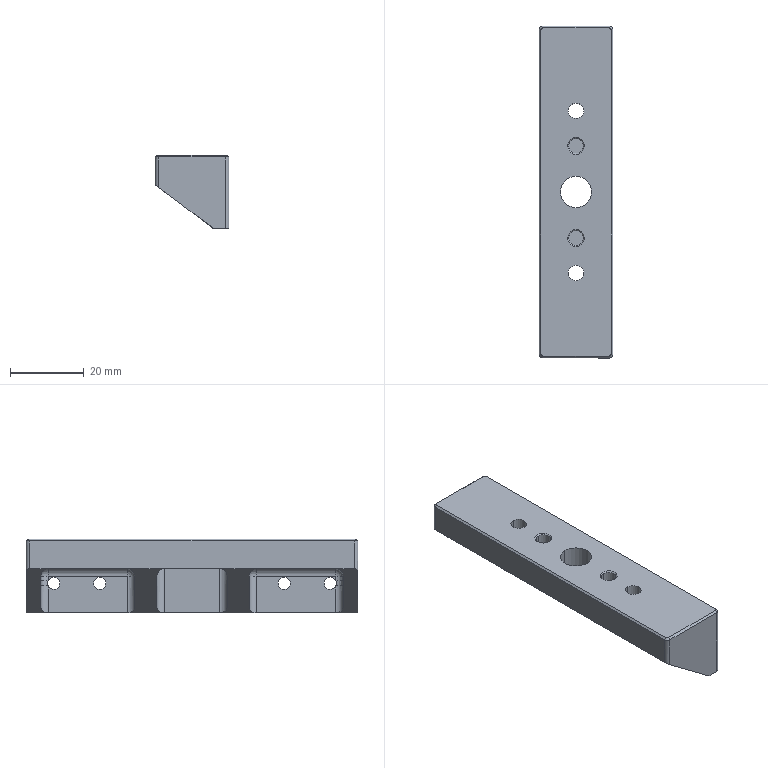NC program | NX | posted with a generic post | part box 20 x 90 x 20 mm
Whole program, first 1403 of 1621 lines:
N10 G17 G21 G94 G90
(FLOOR_WALL , TOOL : D80)
N12 T19 M6
N14 G54
N16 G17 G0 G90 X90. Y0. B0. C0. S6500 M3
N18 G43 Z30. H19
N20 Z3.
N22 G94 G1 Z0. F1500.
N24 X87.
N26 X-87.
N28 X-90.
N30 Z3.
N32 G0 Z30.
N34 M5
(DRILLING , TOOL : D6A45)
N36 T01 M6
N38 G54
N40 G17 G0 G90 X-22. Y0. B0. C0. S5000 M3
N42 G43 Z30. H1
N44 G94 G81 G98 Z-1. F350. R3.
N46 X-12.5
N48 X0.
N50 X12.5
N52 X22.
N54 G80
N56 G0 X22. Y0. Z30.
N58 M5
(DRILLING_COPY_COPY , TOOL : 4.2ZT)
N60 T04 M6
N62 G54
N64 G17 G0 G90 X-22. Y0. B0. C0. S2000 M3
N66 G43 Z30. H4
N68 G94 G83 G98 Z-10.762 F300. Q2. R3.
N70 X22.
N72 G80
N74 G0 X22. Y0. Z30.
N76 M5
(DRILLING_COPY_COPY_1_COPY , TOOL : 3.8ZT)
N78 T18 M6
N80 G54
N82 G17 G0 G90 X12.5 Y0. B0. C0. S2000 M3
N84 G43 Z30. H18
N86 G94 G83 G98 Z-7.142 F200. Q2. R3.
N88 X-12.5
N90 G80
N92 G0 X-12.5 Y0. Z30.
N94 M5
(DRILLING_COPY_COPY_COPY , TOOL : 8.5ZT)
N96 T16 M6
N98 G54
N100 G17 G0 G90 X0. Y0. B0. C0. S2000 M3
N102 G43 Z30. H16
N104 G94 G83 G98 Z-12.054 F300. Q2. R3.
N106 G80
N108 G0 X0. Y0. Z30.
N110 M5
(ZLEVEL_PROFILE , TOOL : D10)
N112 T15 M6
N114 G54
N116 G17 G0 G90 X47.475 Y-14.013 B0. C0. S9500 M3
N118 G43 Z30. H15
N120 Z1.5
N122 G94 G1 X46.237 Y-14.707 Z1.426 F1000.
N124 X44.606 Y-15.1 Z1.338
N126 X0. Z-1.
N128 X-44. F3000.
N130 G2 X-50.1 Y-9. R6.1
N132 G1 Y9.
N134 G2 X-44. Y15.1 R6.1
N136 G1 X44.
N138 G2 X50.1 Y9. R6.1
N140 G1 Y-9.
N142 G2 X44. Y-15.1 R6.1
N144 G1 X0.
N146 X-44. Z-1.176
N148 X-44.598 Y-15.071 Z-1.178
N150 X-45.19 Y-14.983 Z-1.181
N152 X-45.771 Y-14.837 Z-1.183
N154 X-46.334 Y-14.636 Z-1.185
N156 X-46.876 Y-14.38 Z-1.188
N158 X-47.389 Y-14.072 Z-1.19
N160 X-47.87 Y-13.715 Z-1.193
N162 X-48.313 Y-13.313 Z-1.195
N164 X-48.715 Y-12.87 Z-1.197
N166 X-49.072 Y-12.389 Z-1.2
N168 X-49.38 Y-11.876 Z-1.202
N170 X-49.636 Y-11.334 Z-1.204
N172 X-49.837 Y-10.771 Z-1.207
N174 X-49.983 Y-10.19 Z-1.209
N176 X-50.071 Y-9.598 Z-1.212
N178 X-50.1 Y-9. Z-1.214
N180 Y9. Z-1.286
N182 X-50.071 Y9.598 Z-1.288
N184 X-49.983 Y10.19 Z-1.291
N186 X-49.837 Y10.771 Z-1.293
N188 X-49.636 Y11.334 Z-1.296
N190 X-49.38 Y11.876 Z-1.298
N192 X-49.072 Y12.389 Z-1.3
N194 X-48.715 Y12.87 Z-1.303
N196 X-48.313 Y13.313 Z-1.305
N198 X-47.87 Y13.715 Z-1.307
N200 X-47.389 Y14.072 Z-1.31
N202 X-46.876 Y14.38 Z-1.312
N204 X-46.334 Y14.636 Z-1.315
N206 X-45.771 Y14.837 Z-1.317
N208 X-45.19 Y14.983 Z-1.319
N210 X-44.598 Y15.071 Z-1.322
N212 X-44. Y15.1 Z-1.324
N214 X34.222 Z-1.637
N216 X39.111 Z-1.656
N218 X44. Z-1.676
N220 X44.598 Y15.071 Z-1.678
N222 X45.19 Y14.983 Z-1.681
N224 X45.771 Y14.837 Z-1.683
N226 X46.334 Y14.636 Z-1.685
N228 X46.876 Y14.38 Z-1.688
N230 X47.389 Y14.072 Z-1.69
N232 X47.87 Y13.715 Z-1.693
N234 X48.313 Y13.313 Z-1.695
N236 X48.715 Y12.87 Z-1.697
N238 X49.072 Y12.389 Z-1.7
N240 X49.38 Y11.876 Z-1.702
N242 X49.636 Y11.334 Z-1.704
N244 X49.837 Y10.771 Z-1.707
N246 X49.983 Y10.19 Z-1.709
N248 X50.071 Y9.598 Z-1.712
N250 X50.1 Y9. Z-1.714
N252 Y-9. Z-1.786
N254 X50.071 Y-9.598 Z-1.788
N256 X49.983 Y-10.19 Z-1.791
N258 X49.837 Y-10.771 Z-1.793
N260 X49.636 Y-11.334 Z-1.796
N262 X49.38 Y-11.876 Z-1.798
N264 X49.072 Y-12.389 Z-1.8
N266 X48.715 Y-12.87 Z-1.803
N268 X48.313 Y-13.313 Z-1.805
N270 X47.87 Y-13.715 Z-1.807
N272 X47.389 Y-14.072 Z-1.81
N274 X46.876 Y-14.38 Z-1.812
N276 X46.334 Y-14.636 Z-1.815
N278 X45.771 Y-14.837 Z-1.817
N280 X45.19 Y-14.983 Z-1.819
N282 X44.598 Y-15.071 Z-1.822
N284 X44. Y-15.1 Z-1.824
N286 X0. Z-2.
N288 X-44. Z-2.176
N290 X-44.598 Y-15.071 Z-2.178
N292 X-45.19 Y-14.983 Z-2.181
N294 X-45.771 Y-14.837 Z-2.183
N296 X-46.334 Y-14.636 Z-2.185
N298 X-46.876 Y-14.38 Z-2.188
N300 X-47.389 Y-14.072 Z-2.19
N302 X-47.87 Y-13.715 Z-2.193
N304 X-48.313 Y-13.313 Z-2.195
N306 X-48.715 Y-12.87 Z-2.197
N308 X-49.072 Y-12.389 Z-2.2
N310 X-49.38 Y-11.876 Z-2.202
N312 X-49.636 Y-11.334 Z-2.204
N314 X-49.837 Y-10.771 Z-2.207
N316 X-49.983 Y-10.19 Z-2.209
N318 X-50.071 Y-9.598 Z-2.212
N320 X-50.1 Y-9. Z-2.214
N322 Y9. Z-2.286
N324 X-50.071 Y9.598 Z-2.288
N326 X-49.983 Y10.19 Z-2.291
N328 X-49.837 Y10.771 Z-2.293
N330 X-49.636 Y11.334 Z-2.296
N332 X-49.38 Y11.876 Z-2.298
N334 X-49.072 Y12.389 Z-2.3
N336 X-48.715 Y12.87 Z-2.303
N338 X-48.313 Y13.313 Z-2.305
N340 X-47.87 Y13.715 Z-2.307
N342 X-47.389 Y14.072 Z-2.31
N344 X-46.876 Y14.38 Z-2.312
N346 X-46.334 Y14.636 Z-2.315
N348 X-45.771 Y14.837 Z-2.317
N350 X-45.19 Y14.983 Z-2.319
N352 X-44.598 Y15.071 Z-2.322
N354 X-44. Y15.1 Z-2.324
N356 X34.222 Z-2.637
N358 X39.111 Z-2.656
N360 X44. Z-2.676
N362 X44.598 Y15.071 Z-2.678
N364 X45.19 Y14.983 Z-2.681
N366 X45.771 Y14.837 Z-2.683
N368 X46.334 Y14.636 Z-2.685
N370 X46.876 Y14.38 Z-2.688
N372 X47.389 Y14.072 Z-2.69
N374 X47.87 Y13.715 Z-2.693
N376 X48.313 Y13.313 Z-2.695
N378 X48.715 Y12.87 Z-2.697
N380 X49.072 Y12.389 Z-2.7
N382 X49.38 Y11.876 Z-2.702
N384 X49.636 Y11.334 Z-2.704
N386 X49.837 Y10.771 Z-2.707
N388 X49.983 Y10.19 Z-2.709
N390 X50.071 Y9.598 Z-2.712
N392 X50.1 Y9. Z-2.714
N394 Y-9. Z-2.786
N396 X50.071 Y-9.598 Z-2.788
N398 X49.983 Y-10.19 Z-2.791
N400 X49.837 Y-10.771 Z-2.793
N402 X49.636 Y-11.334 Z-2.796
N404 X49.38 Y-11.876 Z-2.798
N406 X49.072 Y-12.389 Z-2.8
N408 X48.715 Y-12.87 Z-2.803
N410 X48.313 Y-13.313 Z-2.805
N412 X47.87 Y-13.715 Z-2.807
N414 X47.389 Y-14.072 Z-2.81
N416 X46.876 Y-14.38 Z-2.812
N418 X46.334 Y-14.636 Z-2.815
N420 X45.771 Y-14.837 Z-2.817
N422 X45.19 Y-14.983 Z-2.819
N424 X44.598 Y-15.071 Z-2.822
N426 X44. Y-15.1 Z-2.824
N428 X0. Z-3.
N430 X-44. Z-3.176
N432 X-44.598 Y-15.071 Z-3.178
N434 X-45.19 Y-14.983 Z-3.181
N436 X-45.771 Y-14.837 Z-3.183
N438 X-46.334 Y-14.636 Z-3.185
N440 X-46.876 Y-14.38 Z-3.188
N442 X-47.389 Y-14.072 Z-3.19
N444 X-47.87 Y-13.715 Z-3.193
N446 X-48.313 Y-13.313 Z-3.195
N448 X-48.715 Y-12.87 Z-3.197
N450 X-49.072 Y-12.389 Z-3.2
N452 X-49.38 Y-11.876 Z-3.202
N454 X-49.636 Y-11.334 Z-3.204
N456 X-49.837 Y-10.771 Z-3.207
N458 X-49.983 Y-10.19 Z-3.209
N460 X-50.071 Y-9.598 Z-3.212
N462 X-50.1 Y-9. Z-3.214
N464 Y9. Z-3.286
N466 X-50.071 Y9.598 Z-3.288
N468 X-49.983 Y10.19 Z-3.291
N470 X-49.837 Y10.771 Z-3.293
N472 X-49.636 Y11.334 Z-3.296
N474 X-49.38 Y11.876 Z-3.298
N476 X-49.072 Y12.389 Z-3.3
N478 X-48.715 Y12.87 Z-3.303
N480 X-48.313 Y13.313 Z-3.305
N482 X-47.87 Y13.715 Z-3.307
N484 X-47.389 Y14.072 Z-3.31
N486 X-46.876 Y14.38 Z-3.312
N488 X-46.334 Y14.636 Z-3.315
N490 X-45.771 Y14.837 Z-3.317
N492 X-45.19 Y14.983 Z-3.319
N494 X-44.598 Y15.071 Z-3.322
N496 X-44. Y15.1 Z-3.324
N498 X34.222 Z-3.637
N500 X39.111 Z-3.656
N502 X44. Z-3.676
N504 X44.598 Y15.071 Z-3.678
N506 X45.19 Y14.983 Z-3.681
N508 X45.771 Y14.837 Z-3.683
N510 X46.334 Y14.636 Z-3.685
N512 X46.876 Y14.38 Z-3.688
N514 X47.389 Y14.072 Z-3.69
N516 X47.87 Y13.715 Z-3.693
N518 X48.313 Y13.313 Z-3.695
N520 X48.715 Y12.87 Z-3.697
N522 X49.072 Y12.389 Z-3.7
N524 X49.38 Y11.876 Z-3.702
N526 X49.636 Y11.334 Z-3.704
N528 X49.837 Y10.771 Z-3.707
N530 X49.983 Y10.19 Z-3.709
N532 X50.071 Y9.598 Z-3.712
N534 X50.1 Y9. Z-3.714
N536 Y-9. Z-3.786
N538 X50.071 Y-9.598 Z-3.788
N540 X49.983 Y-10.19 Z-3.791
N542 X49.837 Y-10.771 Z-3.793
N544 X49.636 Y-11.334 Z-3.796
N546 X49.38 Y-11.876 Z-3.798
N548 X49.072 Y-12.389 Z-3.8
N550 X48.715 Y-12.87 Z-3.803
N552 X48.313 Y-13.313 Z-3.805
N554 X47.87 Y-13.715 Z-3.807
N556 X47.389 Y-14.072 Z-3.81
N558 X46.876 Y-14.38 Z-3.812
N560 X46.334 Y-14.636 Z-3.815
N562 X45.771 Y-14.837 Z-3.817
N564 X45.19 Y-14.983 Z-3.819
N566 X44.598 Y-15.071 Z-3.822
N568 X44. Y-15.1 Z-3.824
N570 X0. Z-4.
N572 X-44. Z-4.176
N574 X-44.598 Y-15.071 Z-4.178
N576 X-45.19 Y-14.983 Z-4.181
N578 X-45.771 Y-14.837 Z-4.183
N580 X-46.334 Y-14.636 Z-4.185
N582 X-46.876 Y-14.38 Z-4.188
N584 X-47.389 Y-14.072 Z-4.19
N586 X-47.87 Y-13.715 Z-4.193
N588 X-48.313 Y-13.313 Z-4.195
N590 X-48.715 Y-12.87 Z-4.197
N592 X-49.072 Y-12.389 Z-4.2
N594 X-49.38 Y-11.876 Z-4.202
N596 X-49.636 Y-11.334 Z-4.204
N598 X-49.837 Y-10.771 Z-4.207
N600 X-49.983 Y-10.19 Z-4.209
N602 X-50.071 Y-9.598 Z-4.212
N604 X-50.1 Y-9. Z-4.214
N606 Y9. Z-4.286
N608 X-50.071 Y9.598 Z-4.288
N610 X-49.983 Y10.19 Z-4.291
N612 X-49.837 Y10.771 Z-4.293
N614 X-49.636 Y11.334 Z-4.296
N616 X-49.38 Y11.876 Z-4.298
N618 X-49.072 Y12.389 Z-4.3
N620 X-48.715 Y12.87 Z-4.303
N622 X-48.313 Y13.313 Z-4.305
N624 X-47.87 Y13.715 Z-4.307
N626 X-47.389 Y14.072 Z-4.31
N628 X-46.876 Y14.38 Z-4.312
N630 X-46.334 Y14.636 Z-4.315
N632 X-45.771 Y14.837 Z-4.317
N634 X-45.19 Y14.983 Z-4.319
N636 X-44.598 Y15.071 Z-4.322
N638 X-44. Y15.1 Z-4.324
N640 X34.222 Z-4.637
N642 X39.111 Z-4.656
N644 X44. Z-4.676
N646 X44.598 Y15.071 Z-4.678
N648 X45.19 Y14.983 Z-4.681
N650 X45.771 Y14.837 Z-4.683
N652 X46.334 Y14.636 Z-4.685
N654 X46.876 Y14.38 Z-4.688
N656 X47.389 Y14.072 Z-4.69
N658 X47.87 Y13.715 Z-4.693
N660 X48.313 Y13.313 Z-4.695
N662 X48.715 Y12.87 Z-4.697
N664 X49.072 Y12.389 Z-4.7
N666 X49.38 Y11.876 Z-4.702
N668 X49.636 Y11.334 Z-4.704
N670 X49.837 Y10.771 Z-4.707
N672 X49.983 Y10.19 Z-4.709
N674 X50.071 Y9.598 Z-4.712
N676 X50.1 Y9. Z-4.714
N678 Y-9. Z-4.786
N680 X50.071 Y-9.598 Z-4.788
N682 X49.983 Y-10.19 Z-4.791
N684 X49.837 Y-10.771 Z-4.793
N686 X49.636 Y-11.334 Z-4.796
N688 X49.38 Y-11.876 Z-4.798
N690 X49.072 Y-12.389 Z-4.8
N692 X48.715 Y-12.87 Z-4.803
N694 X48.313 Y-13.313 Z-4.805
N696 X47.87 Y-13.715 Z-4.807
N698 X47.389 Y-14.072 Z-4.81
N700 X46.876 Y-14.38 Z-4.812
N702 X46.334 Y-14.636 Z-4.815
N704 X45.771 Y-14.837 Z-4.817
N706 X45.19 Y-14.983 Z-4.819
N708 X44.598 Y-15.071 Z-4.822
N710 X44. Y-15.1 Z-4.824
N712 X0. Z-5.
N714 X-44. Z-5.176
N716 X-44.598 Y-15.071 Z-5.178
N718 X-45.19 Y-14.983 Z-5.181
N720 X-45.771 Y-14.837 Z-5.183
N722 X-46.334 Y-14.636 Z-5.185
N724 X-46.876 Y-14.38 Z-5.188
N726 X-47.389 Y-14.072 Z-5.19
N728 X-47.87 Y-13.715 Z-5.193
N730 X-48.313 Y-13.313 Z-5.195
N732 X-48.715 Y-12.87 Z-5.197
N734 X-49.072 Y-12.389 Z-5.2
N736 X-49.38 Y-11.876 Z-5.202
N738 X-49.636 Y-11.334 Z-5.204
N740 X-49.837 Y-10.771 Z-5.207
N742 X-49.983 Y-10.19 Z-5.209
N744 X-50.071 Y-9.598 Z-5.212
N746 X-50.1 Y-9. Z-5.214
N748 Y9. Z-5.286
N750 X-50.071 Y9.598 Z-5.288
N752 X-49.983 Y10.19 Z-5.291
N754 X-49.837 Y10.771 Z-5.293
N756 X-49.636 Y11.334 Z-5.296
N758 X-49.38 Y11.876 Z-5.298
N760 X-49.072 Y12.389 Z-5.3
N762 X-48.715 Y12.87 Z-5.303
N764 X-48.313 Y13.313 Z-5.305
N766 X-47.87 Y13.715 Z-5.307
N768 X-47.389 Y14.072 Z-5.31
N770 X-46.876 Y14.38 Z-5.312
N772 X-46.334 Y14.636 Z-5.315
N774 X-45.771 Y14.837 Z-5.317
N776 X-45.19 Y14.983 Z-5.319
N778 X-44.598 Y15.071 Z-5.322
N780 X-44. Y15.1 Z-5.324
N782 X34.222 Z-5.637
N784 X39.111 Z-5.656
N786 X44. Z-5.676
N788 X44.598 Y15.071 Z-5.678
N790 X45.19 Y14.983 Z-5.681
N792 X45.771 Y14.837 Z-5.683
N794 X46.334 Y14.636 Z-5.685
N796 X46.876 Y14.38 Z-5.688
N798 X47.389 Y14.072 Z-5.69
N800 X47.87 Y13.715 Z-5.693
N802 X48.313 Y13.313 Z-5.695
N804 X48.715 Y12.87 Z-5.697
N806 X49.072 Y12.389 Z-5.7
N808 X49.38 Y11.876 Z-5.702
N810 X49.636 Y11.334 Z-5.704
N812 X49.837 Y10.771 Z-5.707
N814 X49.983 Y10.19 Z-5.709
N816 X50.071 Y9.598 Z-5.712
N818 X50.1 Y9. Z-5.714
N820 Y-9. Z-5.786
N822 X50.071 Y-9.598 Z-5.788
N824 X49.983 Y-10.19 Z-5.791
N826 X49.837 Y-10.771 Z-5.793
N828 X49.636 Y-11.334 Z-5.796
N830 X49.38 Y-11.876 Z-5.798
N832 X49.072 Y-12.389 Z-5.8
N834 X48.715 Y-12.87 Z-5.803
N836 X48.313 Y-13.313 Z-5.805
N838 X47.87 Y-13.715 Z-5.807
N840 X47.389 Y-14.072 Z-5.81
N842 X46.876 Y-14.38 Z-5.812
N844 X46.334 Y-14.636 Z-5.815
N846 X45.771 Y-14.837 Z-5.817
N848 X45.19 Y-14.983 Z-5.819
N850 X44.598 Y-15.071 Z-5.822
N852 X44. Y-15.1 Z-5.824
N854 X0. Z-6.
N856 X-44. Z-6.176
N858 X-44.598 Y-15.071 Z-6.178
N860 X-45.19 Y-14.983 Z-6.181
N862 X-45.771 Y-14.837 Z-6.183
N864 X-46.334 Y-14.636 Z-6.185
N866 X-46.876 Y-14.38 Z-6.188
N868 X-47.389 Y-14.072 Z-6.19
N870 X-47.87 Y-13.715 Z-6.193
N872 X-48.313 Y-13.313 Z-6.195
N874 X-48.715 Y-12.87 Z-6.197
N876 X-49.072 Y-12.389 Z-6.2
N878 X-49.38 Y-11.876 Z-6.202
N880 X-49.636 Y-11.334 Z-6.204
N882 X-49.837 Y-10.771 Z-6.207
N884 X-49.983 Y-10.19 Z-6.209
N886 X-50.071 Y-9.598 Z-6.212
N888 X-50.1 Y-9. Z-6.214
N890 Y9. Z-6.286
N892 X-50.071 Y9.598 Z-6.288
N894 X-49.983 Y10.19 Z-6.291
N896 X-49.837 Y10.771 Z-6.293
N898 X-49.636 Y11.334 Z-6.296
N900 X-49.38 Y11.876 Z-6.298
N902 X-49.072 Y12.389 Z-6.3
N904 X-48.715 Y12.87 Z-6.303
N906 X-48.313 Y13.313 Z-6.305
N908 X-47.87 Y13.715 Z-6.307
N910 X-47.389 Y14.072 Z-6.31
N912 X-46.876 Y14.38 Z-6.312
N914 X-46.334 Y14.636 Z-6.315
N916 X-45.771 Y14.837 Z-6.317
N918 X-45.19 Y14.983 Z-6.319
N920 X-44.598 Y15.071 Z-6.322
N922 X-44. Y15.1 Z-6.324
N924 X34.222 Z-6.637
N926 X39.111 Z-6.656
N928 X44. Z-6.676
N930 X44.598 Y15.071 Z-6.678
N932 X45.19 Y14.983 Z-6.681
N934 X45.771 Y14.837 Z-6.683
N936 X46.334 Y14.636 Z-6.685
N938 X46.876 Y14.38 Z-6.688
N940 X47.389 Y14.072 Z-6.69
N942 X47.87 Y13.715 Z-6.693
N944 X48.313 Y13.313 Z-6.695
N946 X48.715 Y12.87 Z-6.697
N948 X49.072 Y12.389 Z-6.7
N950 X49.38 Y11.876 Z-6.702
N952 X49.636 Y11.334 Z-6.704
N954 X49.837 Y10.771 Z-6.707
N956 X49.983 Y10.19 Z-6.709
N958 X50.071 Y9.598 Z-6.712
N960 X50.1 Y9. Z-6.714
N962 Y-9. Z-6.786
N964 X50.071 Y-9.598 Z-6.788
N966 X49.983 Y-10.19 Z-6.791
N968 X49.837 Y-10.771 Z-6.793
N970 X49.636 Y-11.334 Z-6.796
N972 X49.38 Y-11.876 Z-6.798
N974 X49.072 Y-12.389 Z-6.8
N976 X48.715 Y-12.87 Z-6.803
N978 X48.313 Y-13.313 Z-6.805
N980 X47.87 Y-13.715 Z-6.807
N982 X47.389 Y-14.072 Z-6.81
N984 X46.876 Y-14.38 Z-6.812
N986 X46.334 Y-14.636 Z-6.815
N988 X45.771 Y-14.837 Z-6.817
N990 X45.19 Y-14.983 Z-6.819
N992 X44.598 Y-15.071 Z-6.822
N994 X44. Y-15.1 Z-6.824
N996 X0. Z-7.
N998 X-44. Z-7.176
N1000 X-44.598 Y-15.071 Z-7.178
N1002 X-45.19 Y-14.983 Z-7.181
N1004 X-45.771 Y-14.837 Z-7.183
N1006 X-46.334 Y-14.636 Z-7.185
N1008 X-46.876 Y-14.38 Z-7.188
N1010 X-47.389 Y-14.072 Z-7.19
N1012 X-47.87 Y-13.715 Z-7.193
N1014 X-48.313 Y-13.313 Z-7.195
N1016 X-48.715 Y-12.87 Z-7.197
N1018 X-49.072 Y-12.389 Z-7.2
N1020 X-49.38 Y-11.876 Z-7.202
N1022 X-49.636 Y-11.334 Z-7.204
N1024 X-49.837 Y-10.771 Z-7.207
N1026 X-49.983 Y-10.19 Z-7.209
N1028 X-50.071 Y-9.598 Z-7.212
N1030 X-50.1 Y-9. Z-7.214
N1032 Y9. Z-7.286
N1034 X-50.071 Y9.598 Z-7.288
N1036 X-49.983 Y10.19 Z-7.291
N1038 X-49.837 Y10.771 Z-7.293
N1040 X-49.636 Y11.334 Z-7.296
N1042 X-49.38 Y11.876 Z-7.298
N1044 X-49.072 Y12.389 Z-7.3
N1046 X-48.715 Y12.87 Z-7.303
N1048 X-48.313 Y13.313 Z-7.305
N1050 X-47.87 Y13.715 Z-7.307
N1052 X-47.389 Y14.072 Z-7.31
N1054 X-46.876 Y14.38 Z-7.312
N1056 X-46.334 Y14.636 Z-7.315
N1058 X-45.771 Y14.837 Z-7.317
N1060 X-45.19 Y14.983 Z-7.319
N1062 X-44.598 Y15.071 Z-7.322
N1064 X-44. Y15.1 Z-7.324
N1066 X34.222 Z-7.637
N1068 X39.111 Z-7.656
N1070 X44. Z-7.676
N1072 X44.598 Y15.071 Z-7.678
N1074 X45.19 Y14.983 Z-7.681
N1076 X45.771 Y14.837 Z-7.683
N1078 X46.334 Y14.636 Z-7.685
N1080 X46.876 Y14.38 Z-7.688
N1082 X47.389 Y14.072 Z-7.69
N1084 X47.87 Y13.715 Z-7.693
N1086 X48.313 Y13.313 Z-7.695
N1088 X48.715 Y12.87 Z-7.697
N1090 X49.072 Y12.389 Z-7.7
N1092 X49.38 Y11.876 Z-7.702
N1094 X49.636 Y11.334 Z-7.704
N1096 X49.837 Y10.771 Z-7.707
N1098 X49.983 Y10.19 Z-7.709
N1100 X50.071 Y9.598 Z-7.712
N1102 X50.1 Y9. Z-7.714
N1104 Y-9. Z-7.786
N1106 X50.071 Y-9.598 Z-7.788
N1108 X49.983 Y-10.19 Z-7.791
N1110 X49.837 Y-10.771 Z-7.793
N1112 X49.636 Y-11.334 Z-7.796
N1114 X49.38 Y-11.876 Z-7.798
N1116 X49.072 Y-12.389 Z-7.8
N1118 X48.715 Y-12.87 Z-7.803
N1120 X48.313 Y-13.313 Z-7.805
N1122 X47.87 Y-13.715 Z-7.807
N1124 X47.389 Y-14.072 Z-7.81
N1126 X46.876 Y-14.38 Z-7.812
N1128 X46.334 Y-14.636 Z-7.815
N1130 X45.771 Y-14.837 Z-7.817
N1132 X45.19 Y-14.983 Z-7.819
N1134 X44.598 Y-15.071 Z-7.822
N1136 X44. Y-15.1 Z-7.824
N1138 X0. Z-8.
N1140 X-44. Z-8.176
N1142 X-44.598 Y-15.071 Z-8.178
N1144 X-45.19 Y-14.983 Z-8.181
N1146 X-45.771 Y-14.837 Z-8.183
N1148 X-46.334 Y-14.636 Z-8.185
N1150 X-46.876 Y-14.38 Z-8.188
N1152 X-47.389 Y-14.072 Z-8.19
N1154 X-47.87 Y-13.715 Z-8.193
N1156 X-48.313 Y-13.313 Z-8.195
N1158 X-48.715 Y-12.87 Z-8.197
N1160 X-49.072 Y-12.389 Z-8.2
N1162 X-49.38 Y-11.876 Z-8.202
N1164 X-49.636 Y-11.334 Z-8.204
N1166 X-49.837 Y-10.771 Z-8.207
N1168 X-49.983 Y-10.19 Z-8.209
N1170 X-50.071 Y-9.598 Z-8.212
N1172 X-50.1 Y-9. Z-8.214
N1174 Y9. Z-8.286
N1176 X-50.071 Y9.598 Z-8.288
N1178 X-49.983 Y10.19 Z-8.291
N1180 X-49.837 Y10.771 Z-8.293
N1182 X-49.636 Y11.334 Z-8.296
N1184 X-49.38 Y11.876 Z-8.298
N1186 X-49.072 Y12.389 Z-8.3
N1188 X-48.715 Y12.87 Z-8.303
N1190 X-48.313 Y13.313 Z-8.305
N1192 X-47.87 Y13.715 Z-8.307
N1194 X-47.389 Y14.072 Z-8.31
N1196 X-46.876 Y14.38 Z-8.312
N1198 X-46.334 Y14.636 Z-8.315
N1200 X-45.771 Y14.837 Z-8.317
N1202 X-45.19 Y14.983 Z-8.319
N1204 X-44.598 Y15.071 Z-8.322
N1206 X-44. Y15.1 Z-8.324
N1208 X34.222 Z-8.637
N1210 X39.111 Z-8.656
N1212 X44. Z-8.676
N1214 X44.598 Y15.071 Z-8.678
N1216 X45.19 Y14.983 Z-8.681
N1218 X45.771 Y14.837 Z-8.683
N1220 X46.334 Y14.636 Z-8.685
N1222 X46.876 Y14.38 Z-8.688
N1224 X47.389 Y14.072 Z-8.69
N1226 X47.87 Y13.715 Z-8.693
N1228 X48.313 Y13.313 Z-8.695
N1230 X48.715 Y12.87 Z-8.697
N1232 X49.072 Y12.389 Z-8.7
N1234 X49.38 Y11.876 Z-8.702
N1236 X49.636 Y11.334 Z-8.704
N1238 X49.837 Y10.771 Z-8.707
N1240 X49.983 Y10.19 Z-8.709
N1242 X50.071 Y9.598 Z-8.712
N1244 X50.1 Y9. Z-8.714
N1246 Y-9. Z-8.786
N1248 X50.071 Y-9.598 Z-8.788
N1250 X49.983 Y-10.19 Z-8.791
N1252 X49.837 Y-10.771 Z-8.793
N1254 X49.636 Y-11.334 Z-8.796
N1256 X49.38 Y-11.876 Z-8.798
N1258 X49.072 Y-12.389 Z-8.8
N1260 X48.715 Y-12.87 Z-8.803
N1262 X48.313 Y-13.313 Z-8.805
N1264 X47.87 Y-13.715 Z-8.807
N1266 X47.389 Y-14.072 Z-8.81
N1268 X46.876 Y-14.38 Z-8.812
N1270 X46.334 Y-14.636 Z-8.815
N1272 X45.771 Y-14.837 Z-8.817
N1274 X45.19 Y-14.983 Z-8.819
N1276 X44.598 Y-15.071 Z-8.822
N1278 X44. Y-15.1 Z-8.824
N1280 X0. Z-9.
N1282 X-44. Z-9.176
N1284 X-44.598 Y-15.071 Z-9.178
N1286 X-45.19 Y-14.983 Z-9.181
N1288 X-45.771 Y-14.837 Z-9.183
N1290 X-46.334 Y-14.636 Z-9.185
N1292 X-46.876 Y-14.38 Z-9.188
N1294 X-47.389 Y-14.072 Z-9.19
N1296 X-47.87 Y-13.715 Z-9.193
N1298 X-48.313 Y-13.313 Z-9.195
N1300 X-48.715 Y-12.87 Z-9.197
N1302 X-49.072 Y-12.389 Z-9.2
N1304 X-49.38 Y-11.876 Z-9.202
N1306 X-49.636 Y-11.334 Z-9.204
N1308 X-49.837 Y-10.771 Z-9.207
N1310 X-49.983 Y-10.19 Z-9.209
N1312 X-50.071 Y-9.598 Z-9.212
N1314 X-50.1 Y-9. Z-9.214
N1316 Y9. Z-9.286
N1318 X-50.071 Y9.598 Z-9.288
N1320 X-49.983 Y10.19 Z-9.291
N1322 X-49.837 Y10.771 Z-9.293
N1324 X-49.636 Y11.334 Z-9.296
N1326 X-49.38 Y11.876 Z-9.298
N1328 X-49.072 Y12.389 Z-9.3
N1330 X-48.715 Y12.87 Z-9.303
N1332 X-48.313 Y13.313 Z-9.305
N1334 X-47.87 Y13.715 Z-9.307
N1336 X-47.389 Y14.072 Z-9.31
N1338 X-46.876 Y14.38 Z-9.312
N1340 X-46.334 Y14.636 Z-9.315
N1342 X-45.771 Y14.837 Z-9.317
N1344 X-45.19 Y14.983 Z-9.319
N1346 X-44.598 Y15.071 Z-9.322
N1348 X-44. Y15.1 Z-9.324
N1350 X34.222 Z-9.637
N1352 X39.111 Z-9.656
N1354 X44. Z-9.676
N1356 X44.598 Y15.071 Z-9.678
N1358 X45.19 Y14.983 Z-9.681
N1360 X45.771 Y14.837 Z-9.683
N1362 X46.334 Y14.636 Z-9.685
N1364 X46.876 Y14.38 Z-9.688
N1366 X47.389 Y14.072 Z-9.69
N1368 X47.87 Y13.715 Z-9.693
N1370 X48.313 Y13.313 Z-9.695
N1372 X48.715 Y12.87 Z-9.697
N1374 X49.072 Y12.389 Z-9.7
N1376 X49.38 Y11.876 Z-9.702
N1378 X49.636 Y11.334 Z-9.704
N1380 X49.837 Y10.771 Z-9.707
N1382 X49.983 Y10.19 Z-9.709
N1384 X50.071 Y9.598 Z-9.712
N1386 X50.1 Y9. Z-9.714
N1388 Y-9. Z-9.786
N1390 X50.071 Y-9.598 Z-9.788
N1392 X49.983 Y-10.19 Z-9.791
N1394 X49.837 Y-10.771 Z-9.793
N1396 X49.636 Y-11.334 Z-9.796
N1398 X49.38 Y-11.876 Z-9.798
N1400 X49.072 Y-12.389 Z-9.8
N1402 X48.715 Y-12.87 Z-9.803
N1404 X48.313 Y-13.313 Z-9.805
N1406 X47.87 Y-13.715 Z-9.807
N1408 X47.389 Y-14.072 Z-9.81
N1410 X46.876 Y-14.38 Z-9.812
N1412 X46.334 Y-14.636 Z-9.815
N1414 X45.771 Y-14.837 Z-9.817
N1416 X45.19 Y-14.983 Z-9.819
N1418 X44.598 Y-15.071 Z-9.822
N1420 X44. Y-15.1 Z-9.824
N1422 X0. Z-10.
N1424 X-44. Z-10.176
N1426 X-44.598 Y-15.071 Z-10.178
N1428 X-45.19 Y-14.983 Z-10.181
N1430 X-45.771 Y-14.837 Z-10.183
N1432 X-46.334 Y-14.636 Z-10.185
N1434 X-46.876 Y-14.38 Z-10.188
N1436 X-47.389 Y-14.072 Z-10.19
N1438 X-47.87 Y-13.715 Z-10.193
N1440 X-48.313 Y-13.313 Z-10.195
N1442 X-48.715 Y-12.87 Z-10.197
N1444 X-49.072 Y-12.389 Z-10.2
N1446 X-49.38 Y-11.876 Z-10.202
N1448 X-49.636 Y-11.334 Z-10.204
N1450 X-49.837 Y-10.771 Z-10.207
N1452 X-49.983 Y-10.19 Z-10.209
N1454 X-50.071 Y-9.598 Z-10.212
N1456 X-50.1 Y-9. Z-10.214
N1458 Y9. Z-10.286
N1460 X-50.071 Y9.598 Z-10.288
N1462 X-49.983 Y10.19 Z-10.291
N1464 X-49.837 Y10.771 Z-10.293
N1466 X-49.636 Y11.334 Z-10.296
N1468 X-49.38 Y11.876 Z-10.298
N1470 X-49.072 Y12.389 Z-10.3
N1472 X-48.715 Y12.87 Z-10.303
N1474 X-48.313 Y13.313 Z-10.305
N1476 X-47.87 Y13.715 Z-10.307
N1478 X-47.389 Y14.072 Z-10.31
N1480 X-46.876 Y14.38 Z-10.312
N1482 X-46.334 Y14.636 Z-10.315
N1484 X-45.771 Y14.837 Z-10.317
N1486 X-45.19 Y14.983 Z-10.319
N1488 X-44.598 Y15.071 Z-10.322
N1490 X-44. Y15.1 Z-10.324
N1492 X34.222 Z-10.637
N1494 X39.111 Z-10.656
N1496 X44. Z-10.676
N1498 X44.598 Y15.071 Z-10.678
N1500 X45.19 Y14.983 Z-10.681
N1502 X45.771 Y14.837 Z-10.683
N1504 X46.334 Y14.636 Z-10.685
N1506 X46.876 Y14.38 Z-10.688
N1508 X47.389 Y14.072 Z-10.69
N1510 X47.87 Y13.715 Z-10.693
N1512 X48.313 Y13.313 Z-10.695
N1514 X48.715 Y12.87 Z-10.697
N1516 X49.072 Y12.389 Z-10.7
N1518 X49.38 Y11.876 Z-10.702
N1520 X49.636 Y11.334 Z-10.704
N1522 X49.837 Y10.771 Z-10.707
N1524 X49.983 Y10.19 Z-10.709
N1526 X50.071 Y9.598 Z-10.712
N1528 X50.1 Y9. Z-10.714
N1530 Y-9. Z-10.786
N1532 X50.071 Y-9.598 Z-10.788
N1534 X49.983 Y-10.19 Z-10.791
N1536 X49.837 Y-10.771 Z-10.793
N1538 X49.636 Y-11.334 Z-10.796
N1540 X49.38 Y-11.876 Z-10.798
N1542 X49.072 Y-12.389 Z-10.8
N1544 X48.715 Y-12.87 Z-10.803
N1546 X48.313 Y-13.313 Z-10.805
N1548 X47.87 Y-13.715 Z-10.807
N1550 X47.389 Y-14.072 Z-10.81
N1552 X46.876 Y-14.38 Z-10.812
N1554 X46.334 Y-14.636 Z-10.815
N1556 X45.771 Y-14.837 Z-10.817
N1558 X45.19 Y-14.983 Z-10.819
N1560 X44.598 Y-15.071 Z-10.822
N1562 X44. Y-15.1 Z-10.824
N1564 X0. Z-11.
N1566 X-44. Z-11.176
N1568 X-44.598 Y-15.071 Z-11.178
N1570 X-45.19 Y-14.983 Z-11.181
N1572 X-45.771 Y-14.837 Z-11.183
N1574 X-46.334 Y-14.636 Z-11.185
N1576 X-46.876 Y-14.38 Z-11.188
N1578 X-47.389 Y-14.072 Z-11.19
N1580 X-47.87 Y-13.715 Z-11.193
N1582 X-48.313 Y-13.313 Z-11.195
N1584 X-48.715 Y-12.87 Z-11.197
N1586 X-49.072 Y-12.389 Z-11.2
N1588 X-49.38 Y-11.876 Z-11.202
N1590 X-49.636 Y-11.334 Z-11.204
N1592 X-49.837 Y-10.771 Z-11.207
N1594 X-49.983 Y-10.19 Z-11.209
N1596 X-50.071 Y-9.598 Z-11.212
N1598 X-50.1 Y-9. Z-11.214
N1600 Y9. Z-11.286
N1602 X-50.071 Y9.598 Z-11.288
N1604 X-49.983 Y10.19 Z-11.291
N1606 X-49.837 Y10.771 Z-11.293
N1608 X-49.636 Y11.334 Z-11.296
N1610 X-49.38 Y11.876 Z-11.298
N1612 X-49.072 Y12.389 Z-11.3
N1614 X-48.715 Y12.87 Z-11.303
N1616 X-48.313 Y13.313 Z-11.305
N1618 X-47.87 Y13.715 Z-11.307
N1620 X-47.389 Y14.072 Z-11.31
N1622 X-46.876 Y14.38 Z-11.312
N1624 X-46.334 Y14.636 Z-11.315
N1626 X-45.771 Y14.837 Z-11.317
N1628 X-45.19 Y14.983 Z-11.319
N1630 X-44.598 Y15.071 Z-11.322
N1632 X-44. Y15.1 Z-11.324
N1634 X34.222 Z-11.637
N1636 X39.111 Z-11.656
N1638 X44. Z-11.676
N1640 X44.598 Y15.071 Z-11.678
N1642 X45.19 Y14.983 Z-11.681
N1644 X45.771 Y14.837 Z-11.683
N1646 X46.334 Y14.636 Z-11.685
N1648 X46.876 Y14.38 Z-11.688
N1650 X47.389 Y14.072 Z-11.69
N1652 X47.87 Y13.715 Z-11.693
N1654 X48.313 Y13.313 Z-11.695
N1656 X48.715 Y12.87 Z-11.697
N1658 X49.072 Y12.389 Z-11.7
N1660 X49.38 Y11.876 Z-11.702
N1662 X49.636 Y11.334 Z-11.704
N1664 X49.837 Y10.771 Z-11.707
N1666 X49.983 Y10.19 Z-11.709
N1668 X50.071 Y9.598 Z-11.712
N1670 X50.1 Y9. Z-11.714
N1672 Y-9. Z-11.786
N1674 X50.071 Y-9.598 Z-11.788
N1676 X49.983 Y-10.19 Z-11.791
N1678 X49.837 Y-10.771 Z-11.793
N1680 X49.636 Y-11.334 Z-11.796
N1682 X49.38 Y-11.876 Z-11.798
N1684 X49.072 Y-12.389 Z-11.8
N1686 X48.715 Y-12.87 Z-11.803
N1688 X48.313 Y-13.313 Z-11.805
N1690 X47.87 Y-13.715 Z-11.807
N1692 X47.389 Y-14.072 Z-11.81
N1694 X46.876 Y-14.38 Z-11.812
N1696 X46.334 Y-14.636 Z-11.815
N1698 X45.771 Y-14.837 Z-11.817
N1700 X45.19 Y-14.983 Z-11.819
N1702 X44.598 Y-15.071 Z-11.822
N1704 X44. Y-15.1 Z-11.824
N1706 X0. Z-12.
N1708 X-44. Z-12.176
N1710 X-44.598 Y-15.071 Z-12.178
N1712 X-45.19 Y-14.983 Z-12.181
N1714 X-45.771 Y-14.837 Z-12.183
N1716 X-46.334 Y-14.636 Z-12.185
N1718 X-46.876 Y-14.38 Z-12.188
N1720 X-47.389 Y-14.072 Z-12.19
N1722 X-47.87 Y-13.715 Z-12.193
N1724 X-48.313 Y-13.313 Z-12.195
N1726 X-48.715 Y-12.87 Z-12.197
N1728 X-49.072 Y-12.389 Z-12.2
N1730 X-49.38 Y-11.876 Z-12.202
N1732 X-49.636 Y-11.334 Z-12.204
N1734 X-49.837 Y-10.771 Z-12.207
N1736 X-49.983 Y-10.19 Z-12.209
N1738 X-50.071 Y-9.598 Z-12.212
N1740 X-50.1 Y-9. Z-12.214
N1742 Y9. Z-12.286
N1744 X-50.071 Y9.598 Z-12.288
N1746 X-49.983 Y10.19 Z-12.291
N1748 X-49.837 Y10.771 Z-12.293
N1750 X-49.636 Y11.334 Z-12.296
N1752 X-49.38 Y11.876 Z-12.298
N1754 X-49.072 Y12.389 Z-12.3
N1756 X-48.715 Y12.87 Z-12.303
N1758 X-48.313 Y13.313 Z-12.305
N1760 X-47.87 Y13.715 Z-12.307
N1762 X-47.389 Y14.072 Z-12.31
N1764 X-46.876 Y14.38 Z-12.312
N1766 X-46.334 Y14.636 Z-12.315
N1768 X-45.771 Y14.837 Z-12.317
N1770 X-45.19 Y14.983 Z-12.319
N1772 X-44.598 Y15.071 Z-12.322
N1774 X-44. Y15.1 Z-12.324
N1776 X34.222 Z-12.637
N1778 X39.111 Z-12.656
N1780 X44. Z-12.676
N1782 X44.598 Y15.071 Z-12.678
N1784 X45.19 Y14.983 Z-12.681
N1786 X45.771 Y14.837 Z-12.683
N1788 X46.334 Y14.636 Z-12.685
N1790 X46.876 Y14.38 Z-12.688
N1792 X47.389 Y14.072 Z-12.69
N1794 X47.87 Y13.715 Z-12.693
N1796 X48.313 Y13.313 Z-12.695
N1798 X48.715 Y12.87 Z-12.697
N1800 X49.072 Y12.389 Z-12.7
N1802 X49.38 Y11.876 Z-12.702
N1804 X49.636 Y11.334 Z-12.704
N1806 X49.837 Y10.771 Z-12.707
N1808 X49.983 Y10.19 Z-12.709
N1810 X50.071 Y9.598 Z-12.712
N1812 X50.1 Y9. Z-12.714
N1814 Y-9. Z-12.786
N1816 X50.071 Y-9.598 Z-12.788
N1818 X49.983 Y-10.19 Z-12.791
N1820 X49.837 Y-10.771 Z-12.793
N1822 X49.636 Y-11.334 Z-12.796
N1824 X49.38 Y-11.876 Z-12.798
N1826 X49.072 Y-12.389 Z-12.8
N1828 X48.715 Y-12.87 Z-12.803
N1830 X48.313 Y-13.313 Z-12.805
N1832 X47.87 Y-13.715 Z-12.807
N1834 X47.389 Y-14.072 Z-12.81
N1836 X46.876 Y-14.38 Z-12.812
N1838 X46.334 Y-14.636 Z-12.815
N1840 X45.771 Y-14.837 Z-12.817
N1842 X45.19 Y-14.983 Z-12.819
N1844 X44.598 Y-15.071 Z-12.822
N1846 X44. Y-15.1 Z-12.824
N1848 X0. Z-13.
N1850 X-44. Z-13.176
N1852 X-44.598 Y-15.071 Z-13.178
N1854 X-45.19 Y-14.983 Z-13.181
N1856 X-45.771 Y-14.837 Z-13.183
N1858 X-46.334 Y-14.636 Z-13.185
N1860 X-46.876 Y-14.38 Z-13.188
N1862 X-47.389 Y-14.072 Z-13.19
N1864 X-47.87 Y-13.715 Z-13.193
N1866 X-48.313 Y-13.313 Z-13.195
N1868 X-48.715 Y-12.87 Z-13.197
N1870 X-49.072 Y-12.389 Z-13.2
N1872 X-49.38 Y-11.876 Z-13.202
N1874 X-49.636 Y-11.334 Z-13.204
N1876 X-49.837 Y-10.771 Z-13.207
N1878 X-49.983 Y-10.19 Z-13.209
N1880 X-50.071 Y-9.598 Z-13.212
N1882 X-50.1 Y-9. Z-13.214
N1884 Y9. Z-13.286
N1886 X-50.071 Y9.598 Z-13.288
N1888 X-49.983 Y10.19 Z-13.291
N1890 X-49.837 Y10.771 Z-13.293
N1892 X-49.636 Y11.334 Z-13.296
N1894 X-49.38 Y11.876 Z-13.298
N1896 X-49.072 Y12.389 Z-13.3
N1898 X-48.715 Y12.87 Z-13.303
N1900 X-48.313 Y13.313 Z-13.305
N1902 X-47.87 Y13.715 Z-13.307
N1904 X-47.389 Y14.072 Z-13.31
N1906 X-46.876 Y14.38 Z-13.312
N1908 X-46.334 Y14.636 Z-13.315
N1910 X-45.771 Y14.837 Z-13.317
N1912 X-45.19 Y14.983 Z-13.319
N1914 X-44.598 Y15.071 Z-13.322
N1916 X-44. Y15.1 Z-13.324
N1918 X34.222 Z-13.637
N1920 X39.111 Z-13.656
N1922 X44. Z-13.676
N1924 X44.598 Y15.071 Z-13.678
N1926 X45.19 Y14.983 Z-13.681
N1928 X45.771 Y14.837 Z-13.683
N1930 X46.334 Y14.636 Z-13.685
N1932 X46.876 Y14.38 Z-13.688
N1934 X47.389 Y14.072 Z-13.69
N1936 X47.87 Y13.715 Z-13.693
N1938 X48.313 Y13.313 Z-13.695
N1940 X48.715 Y12.87 Z-13.697
N1942 X49.072 Y12.389 Z-13.7
N1944 X49.38 Y11.876 Z-13.702
N1946 X49.636 Y11.334 Z-13.704
N1948 X49.837 Y10.771 Z-13.707
N1950 X49.983 Y10.19 Z-13.709
N1952 X50.071 Y9.598 Z-13.712
N1954 X50.1 Y9. Z-13.714
N1956 Y-9. Z-13.786
N1958 X50.071 Y-9.598 Z-13.788
N1960 X49.983 Y-10.19 Z-13.791
N1962 X49.837 Y-10.771 Z-13.793
N1964 X49.636 Y-11.334 Z-13.796
N1966 X49.38 Y-11.876 Z-13.798
N1968 X49.072 Y-12.389 Z-13.8
N1970 X48.715 Y-12.87 Z-13.803
N1972 X48.313 Y-13.313 Z-13.805
N1974 X47.87 Y-13.715 Z-13.807
N1976 X47.389 Y-14.072 Z-13.81
N1978 X46.876 Y-14.38 Z-13.812
N1980 X46.334 Y-14.636 Z-13.815
N1982 X45.771 Y-14.837 Z-13.817
N1984 X45.19 Y-14.983 Z-13.819
N1986 X44.598 Y-15.071 Z-13.822
N1988 X44. Y-15.1 Z-13.824
N1990 X0. Z-14.
N1992 X-44. Z-14.176
N1994 X-44.598 Y-15.071 Z-14.178
N1996 X-45.19 Y-14.983 Z-14.181
N1998 X-45.771 Y-14.837 Z-14.183
N2000 X-46.334 Y-14.636 Z-14.185
N2002 X-46.876 Y-14.38 Z-14.188
N2004 X-47.389 Y-14.072 Z-14.19
N2006 X-47.87 Y-13.715 Z-14.193
N2008 X-48.313 Y-13.313 Z-14.195
N2010 X-48.715 Y-12.87 Z-14.197
N2012 X-49.072 Y-12.389 Z-14.2
N2014 X-49.38 Y-11.876 Z-14.202
N2016 X-49.636 Y-11.334 Z-14.204
N2018 X-49.837 Y-10.771 Z-14.207
N2020 X-49.983 Y-10.19 Z-14.209
N2022 X-50.071 Y-9.598 Z-14.212
N2024 X-50.1 Y-9. Z-14.214
N2026 Y9. Z-14.286
N2028 X-50.071 Y9.598 Z-14.288
N2030 X-49.983 Y10.19 Z-14.291
N2032 X-49.837 Y10.771 Z-14.293
N2034 X-49.636 Y11.334 Z-14.296
N2036 X-49.38 Y11.876 Z-14.298
N2038 X-49.072 Y12.389 Z-14.3
N2040 X-48.715 Y12.87 Z-14.303
N2042 X-48.313 Y13.313 Z-14.305
N2044 X-47.87 Y13.715 Z-14.307
N2046 X-47.389 Y14.072 Z-14.31
N2048 X-46.876 Y14.38 Z-14.312
N2050 X-46.334 Y14.636 Z-14.315
N2052 X-45.771 Y14.837 Z-14.317
N2054 X-45.19 Y14.983 Z-14.319
N2056 X-44.598 Y15.071 Z-14.322
N2058 X-44. Y15.1 Z-14.324
N2060 X34.222 Z-14.637
N2062 X39.111 Z-14.656
N2064 X44. Z-14.676
N2066 X44.598 Y15.071 Z-14.678
N2068 X45.19 Y14.983 Z-14.681
N2070 X45.771 Y14.837 Z-14.683
N2072 X46.334 Y14.636 Z-14.685
N2074 X46.876 Y14.38 Z-14.688
N2076 X47.389 Y14.072 Z-14.69
N2078 X47.87 Y13.715 Z-14.693
N2080 X48.313 Y13.313 Z-14.695
N2082 X48.715 Y12.87 Z-14.697
N2084 X49.072 Y12.389 Z-14.7
N2086 X49.38 Y11.876 Z-14.702
N2088 X49.636 Y11.334 Z-14.704
N2090 X49.837 Y10.771 Z-14.707
N2092 X49.983 Y10.19 Z-14.709
N2094 X50.071 Y9.598 Z-14.712
N2096 X50.1 Y9. Z-14.714
N2098 Y-9. Z-14.786
N2100 X50.071 Y-9.598 Z-14.788
N2102 X49.983 Y-10.19 Z-14.791
N2104 X49.837 Y-10.771 Z-14.793
N2106 X49.636 Y-11.334 Z-14.796
N2108 X49.38 Y-11.876 Z-14.798
N2110 X49.072 Y-12.389 Z-14.8
N2112 X48.715 Y-12.87 Z-14.803
N2114 X48.313 Y-13.313 Z-14.805
N2116 X47.87 Y-13.715 Z-14.807
N2118 X47.389 Y-14.072 Z-14.81
N2120 X46.876 Y-14.38 Z-14.812
N2122 X46.334 Y-14.636 Z-14.815
N2124 X45.771 Y-14.837 Z-14.817
N2126 X45.19 Y-14.983 Z-14.819
N2128 X44.598 Y-15.071 Z-14.822
N2130 X44. Y-15.1 Z-14.824
N2132 X0. Z-15.
N2134 X-44. Z-15.176
N2136 X-44.598 Y-15.071 Z-15.178
N2138 X-45.19 Y-14.983 Z-15.181
N2140 X-45.771 Y-14.837 Z-15.183
N2142 X-46.334 Y-14.636 Z-15.185
N2144 X-46.876 Y-14.38 Z-15.188
N2146 X-47.389 Y-14.072 Z-15.19
N2148 X-47.87 Y-13.715 Z-15.193
N2150 X-48.313 Y-13.313 Z-15.195
N2152 X-48.715 Y-12.87 Z-15.197
N2154 X-49.072 Y-12.389 Z-15.2
N2156 X-49.38 Y-11.876 Z-15.202
N2158 X-49.636 Y-11.334 Z-15.204
N2160 X-49.837 Y-10.771 Z-15.207
N2162 X-49.983 Y-10.19 Z-15.209
N2164 X-50.071 Y-9.598 Z-15.212
N2166 X-50.1 Y-9. Z-15.214
N2168 Y9. Z-15.286
N2170 X-50.071 Y9.598 Z-15.288
N2172 X-49.983 Y10.19 Z-15.291
N2174 X-49.837 Y10.771 Z-15.293
N2176 X-49.636 Y11.334 Z-15.296
N2178 X-49.38 Y11.876 Z-15.298
N2180 X-49.072 Y12.389 Z-15.3
N2182 X-48.715 Y12.87 Z-15.303
N2184 X-48.313 Y13.313 Z-15.305
N2186 X-47.87 Y13.715 Z-15.307
N2188 X-47.389 Y14.072 Z-15.31
N2190 X-46.876 Y14.38 Z-15.312
N2192 X-46.334 Y14.636 Z-15.315
N2194 X-45.771 Y14.837 Z-15.317
N2196 X-45.19 Y14.983 Z-15.319
N2198 X-44.598 Y15.071 Z-15.322
N2200 X-44. Y15.1 Z-15.324
N2202 X34.222 Z-15.637
N2204 X39.111 Z-15.656
N2206 X44. Z-15.676
N2208 X44.598 Y15.071 Z-15.678
N2210 X45.19 Y14.983 Z-15.681
N2212 X45.771 Y14.837 Z-15.683
N2214 X46.334 Y14.636 Z-15.685
N2216 X46.876 Y14.38 Z-15.688
N2218 X47.389 Y14.072 Z-15.69
N2220 X47.87 Y13.715 Z-15.693
N2222 X48.313 Y13.313 Z-15.695
N2224 X48.715 Y12.87 Z-15.697
N2226 X49.072 Y12.389 Z-15.7
N2228 X49.38 Y11.876 Z-15.702
N2230 X49.636 Y11.334 Z-15.704
N2232 X49.837 Y10.771 Z-15.707
N2234 X49.983 Y10.19 Z-15.709
N2236 X50.071 Y9.598 Z-15.712
N2238 X50.1 Y9. Z-15.714
N2240 Y-9. Z-15.786
N2242 X50.071 Y-9.598 Z-15.788
N2244 X49.983 Y-10.19 Z-15.791
N2246 X49.837 Y-10.771 Z-15.793
N2248 X49.636 Y-11.334 Z-15.796
N2250 X49.38 Y-11.876 Z-15.798
N2252 X49.072 Y-12.389 Z-15.8
N2254 X48.715 Y-12.87 Z-15.803
N2256 X48.313 Y-13.313 Z-15.805
N2258 X47.87 Y-13.715 Z-15.807
N2260 X47.389 Y-14.072 Z-15.81
N2262 X46.876 Y-14.38 Z-15.812
N2264 X46.334 Y-14.636 Z-15.815
N2266 X45.771 Y-14.837 Z-15.817
N2268 X45.19 Y-14.983 Z-15.819
N2270 X44.598 Y-15.071 Z-15.822
N2272 X44. Y-15.1 Z-15.824
N2274 X0. Z-16.
N2276 X-44. Z-16.176
N2278 X-44.598 Y-15.071 Z-16.178
N2280 X-45.19 Y-14.983 Z-16.181
N2282 X-45.771 Y-14.837 Z-16.183
N2284 X-46.334 Y-14.636 Z-16.185
N2286 X-46.876 Y-14.38 Z-16.188
N2288 X-47.389 Y-14.072 Z-16.19
N2290 X-47.87 Y-13.715 Z-16.193
N2292 X-48.313 Y-13.313 Z-16.195
N2294 X-48.715 Y-12.87 Z-16.197
N2296 X-49.072 Y-12.389 Z-16.2
N2298 X-49.38 Y-11.876 Z-16.202
N2300 X-49.636 Y-11.334 Z-16.204
N2302 X-49.837 Y-10.771 Z-16.207
N2304 X-49.983 Y-10.19 Z-16.209
N2306 X-50.071 Y-9.598 Z-16.212
N2308 X-50.1 Y-9. Z-16.214
N2310 Y9. Z-16.286
N2312 X-50.071 Y9.598 Z-16.288
N2314 X-49.983 Y10.19 Z-16.291
N2316 X-49.837 Y10.771 Z-16.293
N2318 X-49.636 Y11.334 Z-16.296
N2320 X-49.38 Y11.876 Z-16.298
N2322 X-49.072 Y12.389 Z-16.3
N2324 X-48.715 Y12.87 Z-16.303
N2326 X-48.313 Y13.313 Z-16.305
N2328 X-47.87 Y13.715 Z-16.307
N2330 X-47.389 Y14.072 Z-16.31
N2332 X-46.876 Y14.38 Z-16.312
N2334 X-46.334 Y14.636 Z-16.315
N2336 X-45.771 Y14.837 Z-16.317
N2338 X-45.19 Y14.983 Z-16.319
N2340 X-44.598 Y15.071 Z-16.322
N2342 X-44. Y15.1 Z-16.324
N2344 X34.222 Z-16.637
N2346 X39.111 Z-16.656
N2348 X44. Z-16.676
N2350 X44.598 Y15.071 Z-16.678
N2352 X45.19 Y14.983 Z-16.681
N2354 X45.771 Y14.837 Z-16.683
N2356 X46.334 Y14.636 Z-16.685
N2358 X46.876 Y14.38 Z-16.688
N2360 X47.389 Y14.072 Z-16.69
N2362 X47.87 Y13.715 Z-16.693
N2364 X48.313 Y13.313 Z-16.695
N2366 X48.715 Y12.87 Z-16.697
N2368 X49.072 Y12.389 Z-16.7
N2370 X49.38 Y11.876 Z-16.702
N2372 X49.636 Y11.334 Z-16.704
N2374 X49.837 Y10.771 Z-16.707
N2376 X49.983 Y10.19 Z-16.709
N2378 X50.071 Y9.598 Z-16.712
N2380 X50.1 Y9. Z-16.714
N2382 Y-9. Z-16.786
N2384 X50.071 Y-9.598 Z-16.788
N2386 X49.983 Y-10.19 Z-16.791
N2388 X49.837 Y-10.771 Z-16.793
N2390 X49.636 Y-11.334 Z-16.796
N2392 X49.38 Y-11.876 Z-16.798
N2394 X49.072 Y-12.389 Z-16.8
N2396 X48.715 Y-12.87 Z-16.803
N2398 X48.313 Y-13.313 Z-16.805
N2400 X47.87 Y-13.715 Z-16.807
N2402 X47.389 Y-14.072 Z-16.81
N2404 X46.876 Y-14.38 Z-16.812
N2406 X46.334 Y-14.636 Z-16.815
N2408 X45.771 Y-14.837 Z-16.817
N2410 X45.19 Y-14.983 Z-16.819
N2412 X44.598 Y-15.071 Z-16.822
N2414 X44. Y-15.1 Z-16.824
N2416 X0. Z-17.
N2418 X-44. Z-17.176
N2420 X-44.598 Y-15.071 Z-17.178
N2422 X-45.19 Y-14.983 Z-17.181
N2424 X-45.771 Y-14.837 Z-17.183
N2426 X-46.334 Y-14.636 Z-17.185
N2428 X-46.876 Y-14.38 Z-17.188
N2430 X-47.389 Y-14.072 Z-17.19
N2432 X-47.87 Y-13.715 Z-17.193
N2434 X-48.313 Y-13.313 Z-17.195
N2436 X-48.715 Y-12.87 Z-17.197
N2438 X-49.072 Y-12.389 Z-17.2
N2440 X-49.38 Y-11.876 Z-17.202
N2442 X-49.636 Y-11.334 Z-17.204
N2444 X-49.837 Y-10.771 Z-17.207
N2446 X-49.983 Y-10.19 Z-17.209
N2448 X-50.071 Y-9.598 Z-17.212
N2450 X-50.1 Y-9. Z-17.214
N2452 Y9. Z-17.286
N2454 X-50.071 Y9.598 Z-17.288
N2456 X-49.983 Y10.19 Z-17.291
N2458 X-49.837 Y10.771 Z-17.293
N2460 X-49.636 Y11.334 Z-17.296
N2462 X-49.38 Y11.876 Z-17.298
N2464 X-49.072 Y12.389 Z-17.3
N2466 X-48.715 Y12.87 Z-17.303
N2468 X-48.313 Y13.313 Z-17.305
N2470 X-47.87 Y13.715 Z-17.307
N2472 X-47.389 Y14.072 Z-17.31
N2474 X-46.876 Y14.38 Z-17.312
N2476 X-46.334 Y14.636 Z-17.315
N2478 X-45.771 Y14.837 Z-17.317
N2480 X-45.19 Y14.983 Z-17.319
N2482 X-44.598 Y15.071 Z-17.322
N2484 X-44. Y15.1 Z-17.324
N2486 X34.222 Z-17.637
N2488 X39.111 Z-17.656
N2490 X44. Z-17.676
N2492 X44.598 Y15.071 Z-17.678
N2494 X45.19 Y14.983 Z-17.681
N2496 X45.771 Y14.837 Z-17.683
N2498 X46.334 Y14.636 Z-17.685
N2500 X46.876 Y14.38 Z-17.688
N2502 X47.389 Y14.072 Z-17.69
N2504 X47.87 Y13.715 Z-17.693
N2506 X48.313 Y13.313 Z-17.695
N2508 X48.715 Y12.87 Z-17.697
N2510 X49.072 Y12.389 Z-17.7
N2512 X49.38 Y11.876 Z-17.702
N2514 X49.636 Y11.334 Z-17.704
N2516 X49.837 Y10.771 Z-17.707
N2518 X49.983 Y10.19 Z-17.709
N2520 X50.071 Y9.598 Z-17.712
N2522 X50.1 Y9. Z-17.714
N2524 Y-9. Z-17.786
N2526 X50.071 Y-9.598 Z-17.788
N2528 X49.983 Y-10.19 Z-17.791
N2530 X49.837 Y-10.771 Z-17.793
N2532 X49.636 Y-11.334 Z-17.796
N2534 X49.38 Y-11.876 Z-17.798
N2536 X49.072 Y-12.389 Z-17.8
N2538 X48.715 Y-12.87 Z-17.803
N2540 X48.313 Y-13.313 Z-17.805
N2542 X47.87 Y-13.715 Z-17.807
N2544 X47.389 Y-14.072 Z-17.81
N2546 X46.876 Y-14.38 Z-17.812
N2548 X46.334 Y-14.636 Z-17.815
N2550 X45.771 Y-14.837 Z-17.817
N2552 X45.19 Y-14.983 Z-17.819
N2554 X44.598 Y-15.071 Z-17.822
N2556 X44. Y-15.1 Z-17.824
N2558 X0. Z-18.
N2560 X-44. Z-18.176
N2562 X-44.598 Y-15.071 Z-18.178
N2564 X-45.19 Y-14.983 Z-18.181
N2566 X-45.771 Y-14.837 Z-18.183
N2568 X-46.334 Y-14.636 Z-18.185
N2570 X-46.876 Y-14.38 Z-18.188
N2572 X-47.389 Y-14.072 Z-18.19
N2574 X-47.87 Y-13.715 Z-18.193
N2576 X-48.313 Y-13.313 Z-18.195
N2578 X-48.715 Y-12.87 Z-18.197
N2580 X-49.072 Y-12.389 Z-18.2
N2582 X-49.38 Y-11.876 Z-18.202
N2584 X-49.636 Y-11.334 Z-18.204
N2586 X-49.837 Y-10.771 Z-18.207
N2588 X-49.983 Y-10.19 Z-18.209
N2590 X-50.071 Y-9.598 Z-18.212
N2592 X-50.1 Y-9. Z-18.214
N2594 Y9. Z-18.286
N2596 X-50.071 Y9.598 Z-18.288
N2598 X-49.983 Y10.19 Z-18.291
N2600 X-49.837 Y10.771 Z-18.293
N2602 X-49.636 Y11.334 Z-18.296
N2604 X-49.38 Y11.876 Z-18.298
N2606 X-49.072 Y12.389 Z-18.3
N2608 X-48.715 Y12.87 Z-18.303
N2610 X-48.313 Y13.313 Z-18.305
N2612 X-47.87 Y13.715 Z-18.307
N2614 X-47.389 Y14.072 Z-18.31
N2616 X-46.876 Y14.38 Z-18.312
N2618 X-46.334 Y14.636 Z-18.315
N2620 X-45.771 Y14.837 Z-18.317
N2622 X-45.19 Y14.983 Z-18.319
N2624 X-44.598 Y15.071 Z-18.322
N2626 X-44. Y15.1 Z-18.324
N2628 X34.222 Z-18.637
N2630 X39.111 Z-18.656
N2632 X44. Z-18.676
N2634 X44.598 Y15.071 Z-18.678
N2636 X45.19 Y14.983 Z-18.681
N2638 X45.771 Y14.837 Z-18.683
N2640 X46.334 Y14.636 Z-18.685
N2642 X46.876 Y14.38 Z-18.688
N2644 X47.389 Y14.072 Z-18.69
N2646 X47.87 Y13.715 Z-18.693
N2648 X48.313 Y13.313 Z-18.695
N2650 X48.715 Y12.87 Z-18.697
N2652 X49.072 Y12.389 Z-18.7
N2654 X49.38 Y11.876 Z-18.702
N2656 X49.636 Y11.334 Z-18.704
N2658 X49.837 Y10.771 Z-18.707
N2660 X49.983 Y10.19 Z-18.709
N2662 X50.071 Y9.598 Z-18.712
N2664 X50.1 Y9. Z-18.714
N2666 Y-9. Z-18.786
N2668 X50.071 Y-9.598 Z-18.788
N2670 X49.983 Y-10.19 Z-18.791
N2672 X49.837 Y-10.771 Z-18.793
N2674 X49.636 Y-11.334 Z-18.796
N2676 X49.38 Y-11.876 Z-18.798
N2678 X49.072 Y-12.389 Z-18.8
N2680 X48.715 Y-12.87 Z-18.803
N2682 X48.313 Y-13.313 Z-18.805
N2684 X47.87 Y-13.715 Z-18.807
N2686 X47.389 Y-14.072 Z-18.81
N2688 X46.876 Y-14.38 Z-18.812
N2690 X46.334 Y-14.636 Z-18.815
N2692 X45.771 Y-14.837 Z-18.817
N2694 X45.19 Y-14.983 Z-18.819
N2696 X44.598 Y-15.071 Z-18.822
N2698 X44. Y-15.1 Z-18.824
N2700 X0. Z-19.
N2702 X-44. Z-19.176
N2704 X-44.598 Y-15.071 Z-19.178
N2706 X-45.19 Y-14.983 Z-19.181
N2708 X-45.771 Y-14.837 Z-19.183
N2710 X-46.334 Y-14.636 Z-19.185
N2712 X-46.876 Y-14.38 Z-19.188
N2714 X-47.389 Y-14.072 Z-19.19
N2716 X-47.87 Y-13.715 Z-19.193
N2718 X-48.313 Y-13.313 Z-19.195
N2720 X-48.715 Y-12.87 Z-19.197
N2722 X-49.072 Y-12.389 Z-19.2
N2724 X-49.38 Y-11.876 Z-19.202
N2726 X-49.636 Y-11.334 Z-19.204
N2728 X-49.837 Y-10.771 Z-19.207
N2730 X-49.983 Y-10.19 Z-19.209
N2732 X-50.071 Y-9.598 Z-19.212
N2734 X-50.1 Y-9. Z-19.214
N2736 Y9. Z-19.286
N2738 X-50.071 Y9.598 Z-19.288
N2740 X-49.983 Y10.19 Z-19.291
N2742 X-49.837 Y10.771 Z-19.293
N2744 X-49.636 Y11.334 Z-19.296
N2746 X-49.38 Y11.876 Z-19.298
N2748 X-49.072 Y12.389 Z-19.3
N2750 X-48.715 Y12.87 Z-19.303
N2752 X-48.313 Y13.313 Z-19.305
N2754 X-47.87 Y13.715 Z-19.307
N2756 X-47.389 Y14.072 Z-19.31
N2758 X-46.876 Y14.38 Z-19.312
N2760 X-46.334 Y14.636 Z-19.315
N2762 X-45.771 Y14.837 Z-19.317
N2764 X-45.19 Y14.983 Z-19.319
N2766 X-44.598 Y15.071 Z-19.322
N2768 X-44. Y15.1 Z-19.324
N2770 X34.222 Z-19.637
N2772 X39.111 Z-19.656
N2774 X44. Z-19.676
N2776 X44.598 Y15.071 Z-19.678
N2778 X45.19 Y14.983 Z-19.681
N2780 X45.771 Y14.837 Z-19.683
N2782 X46.334 Y14.636 Z-19.685
N2784 X46.876 Y14.38 Z-19.688
N2786 X47.389 Y14.072 Z-19.69
N2788 X47.87 Y13.715 Z-19.693
N2790 X48.313 Y13.313 Z-19.695
N2792 X48.715 Y12.87 Z-19.697
N2794 X49.072 Y12.389 Z-19.7
N2796 X49.38 Y11.876 Z-19.702
N2798 X49.636 Y11.334 Z-19.704
N2800 X49.837 Y10.771 Z-19.707
N2802 X49.983 Y10.19 Z-19.709